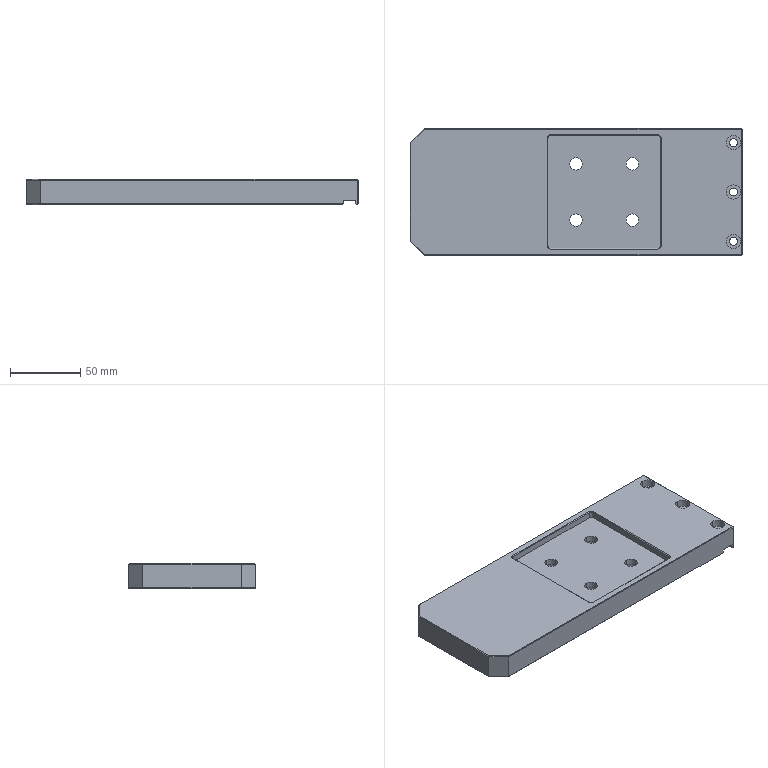NC program | NX | posted with a generic post | part box 235.5 x 90 x 18 mm
Lines 1 to 1608 of 2446:
N10 G17 G21 G94 G90
(DRILLING , TOOL : D6A45)
N12 T01 M6
N14 G54
N16 G17 G0 G90 X111.75 Y35. S5000 M3
N18 G43 Z30. H1
N20 G94 G81 G98 Z-2. F250. R3.
N22 Y0.
N24 Y-35.
N26 X40. Y-20.
N28 X0.
N30 Y20.
N32 X40.
N34 G80
N36 G0 X40. Y20. Z30.
N38 M5
(DRILLING_1 , TOOL : 5.5ZT)
N40 T09 M6
N42 G54
N44 G17 G0 G90 X111.75 Y35. S2000 M3
N46 G43 Z30. H9
N48 G94 G83 G98 Z-21.152 F200. Q2. R3.
N50 Y0.
N52 Y-35.
N54 G80
N56 G0 X111.75 Y-35. Z30.
N58 M5
(DRILLING_1_COPY , TOOL : 9.0ZT)
N60 T16 M6
N62 G54
N64 G17 G0 G90 X0. Y-20. S2000 M3
N66 G43 Z30. H16
N68 G94 G83 G98 Z-22.204 F200. Q2. R3.
N70 Y20.
N72 X40.
N74 Y-20.
N76 G80
N78 G0 X40. Y-20. Z30.
N80 M5
(ZLEVEL_PROFILE , TOOL : D10)
N82 T15 M6
N84 G54
N86 G17 G0 G90 X-122.85 Y10.11 S9500 M3
N88 G43 Z30. H15
N90 Z1.5
N92 G94 G1 Y35.554 Z0.167 F1000.
N94 X-122.49 Y36.963 Z0.09
N96 X-121.748 Y38.215 Z0.014
N98 X-110.965 Y48.998 Z-0.785
N100 X-109.713 Y49.74 Z-0.861
N102 X-108.304 Y50.1 Z-0.938
N104 X-107.75 Z-0.967
N106 X117.25 F3500.
N108 G2 X120.856 Y48.606 R5.1
N110 G1 X121.356 Y48.106
N112 G2 X122.85 Y44.5 R5.1
N114 G1 Y-44.5
N116 G2 X121.356 Y-48.106 R5.1
N118 G1 X120.856 Y-48.606
N120 G2 X117.25 Y-50.1 R5.1
N122 G1 X-107.75
N124 G2 X-111.356 Y-48.606 R5.1
N126 G1 X-121.356 Y-38.606
N128 G2 X-122.85 Y-35. R5.1
N130 G1 Y35.
N132 G2 X-121.356 Y38.606 R5.1
N134 G1 X-111.356 Y48.606
N136 G2 X-107.75 Y50.1 R5.1
N138 G1 X117.25 Z-1.291
N140 X117.75 Y50.075 Z-1.292
N142 X118.245 Y50.002
N144 X118.73 Y49.88 Z-1.293
N146 X119.202 Y49.712 Z-1.294
N148 X119.654 Y49.498 Z-1.295
N150 X120.083 Y49.24
N152 X120.485 Y48.942 Z-1.296
N154 X120.856 Y48.606 Z-1.297
N156 X121.356 Y48.106 Z-1.298
N158 X121.692 Y47.735
N160 X121.99 Y47.333 Z-1.299
N162 X122.248 Y46.904 Z-1.3
N164 X122.462 Y46.452 Z-1.301
N166 X122.63 Y45.98
N168 X122.752 Y45.495 Z-1.302
N170 X122.825 Y45. Z-1.303
N172 X122.85 Y44.5 Z-1.304
N174 Y-44.5 Z-1.432
N176 X122.825 Y-45. Z-1.433
N178 X122.752 Y-45.495
N180 X122.63 Y-45.98 Z-1.434
N182 X122.462 Y-46.452 Z-1.435
N184 X122.248 Y-46.904
N186 X121.99 Y-47.333 Z-1.436
N188 X121.692 Y-47.735 Z-1.437
N190 X121.356 Y-48.106 Z-1.438
N192 X120.856 Y-48.606 Z-1.439
N194 X120.485 Y-48.942
N196 X120.083 Y-49.24 Z-1.44
N198 X119.654 Y-49.498 Z-1.441
N200 X119.202 Y-49.712
N202 X118.73 Y-49.88 Z-1.442
N204 X118.245 Y-50.002 Z-1.443
N206 X117.75 Y-50.075 Z-1.444
N208 X117.25 Y-50.1
N210 X-107.75 Z-1.769
N212 X-108.25 Y-50.075
N214 X-108.745 Y-50.002 Z-1.77
N216 X-109.23 Y-49.88 Z-1.771
N218 X-109.702 Y-49.712 Z-1.772
N220 X-110.154 Y-49.498
N222 X-110.583 Y-49.24 Z-1.773
N224 X-110.985 Y-48.942 Z-1.774
N226 X-111.356 Y-48.606
N228 X-121.356 Y-38.606 Z-1.795
N230 X-121.692 Y-38.235
N232 X-121.99 Y-37.833 Z-1.796
N234 X-122.248 Y-37.404 Z-1.797
N236 X-122.462 Y-36.952 Z-1.798
N238 X-122.63 Y-36.48
N240 X-122.752 Y-35.995 Z-1.799
N242 X-122.825 Y-35.5 Z-1.8
N244 X-122.85 Y-35. Z-1.801
N246 Y35. Z-1.901
N248 X-122.825 Y35.5 Z-1.902
N250 X-122.752 Y35.995 Z-1.903
N252 X-122.63 Y36.48 Z-1.904
N254 X-122.462 Y36.952
N256 X-122.248 Y37.404 Z-1.905
N258 X-121.99 Y37.833 Z-1.906
N260 X-121.692 Y38.235
N262 X-121.356 Y38.606 Z-1.907
N264 X-111.356 Y48.606 Z-1.928
N266 X-110.985 Y48.942
N268 X-110.583 Y49.24 Z-1.929
N270 X-110.154 Y49.498 Z-1.93
N272 X-109.702 Y49.712
N274 X-109.23 Y49.88 Z-1.931
N276 X-108.745 Y50.002 Z-1.932
N278 X-108.25 Y50.075 Z-1.933
N280 X-107.75 Y50.1
N282 X117.25 Z-2.258
N284 X117.75 Y50.075
N286 X118.245 Y50.002 Z-2.259
N288 X118.73 Y49.88 Z-2.26
N290 X119.202 Y49.712 Z-2.261
N292 X119.654 Y49.498
N294 X120.083 Y49.24 Z-2.262
N296 X120.485 Y48.942 Z-2.263
N298 X120.856 Y48.606
N300 X121.356 Y48.106 Z-2.264
N302 X121.692 Y47.735 Z-2.265
N304 X121.99 Y47.333 Z-2.266
N306 X122.248 Y46.904 Z-2.267
N308 X122.462 Y46.452
N310 X122.63 Y45.98 Z-2.268
N312 X122.752 Y45.495 Z-2.269
N314 X122.825 Y45.
N316 X122.85 Y44.5 Z-2.27
N318 Y-44.5 Z-2.398
N320 X122.825 Y-45. Z-2.399
N322 X122.752 Y-45.495 Z-2.4
N324 X122.63 Y-45.98 Z-2.401
N326 X122.462 Y-46.452
N328 X122.248 Y-46.904 Z-2.402
N330 X121.99 Y-47.333 Z-2.403
N332 X121.692 Y-47.735
N334 X121.356 Y-48.106 Z-2.404
N336 X120.856 Y-48.606 Z-2.405
N338 X120.485 Y-48.942 Z-2.406
N340 X120.083 Y-49.24 Z-2.407
N342 X119.654 Y-49.498
N344 X119.202 Y-49.712 Z-2.408
N346 X118.73 Y-49.88 Z-2.409
N348 X118.245 Y-50.002 Z-2.41
N350 X117.75 Y-50.075
N352 X117.25 Y-50.1 Z-2.411
N354 X-107.75 Z-2.735
N356 X-108.25 Y-50.075 Z-2.736
N358 X-108.745 Y-50.002 Z-2.737
N360 X-109.23 Y-49.88
N362 X-109.702 Y-49.712 Z-2.738
N364 X-110.154 Y-49.498 Z-2.739
N366 X-110.583 Y-49.24 Z-2.74
N368 X-110.985 Y-48.942
N370 X-111.356 Y-48.606 Z-2.741
N372 X-121.356 Y-38.606 Z-2.761
N374 X-121.692 Y-38.235 Z-2.762
N376 X-121.99 Y-37.833 Z-2.763
N378 X-122.248 Y-37.404 Z-2.764
N380 X-122.462 Y-36.952
N382 X-122.63 Y-36.48 Z-2.765
N384 X-122.752 Y-35.995 Z-2.766
N386 X-122.825 Y-35.5
N388 X-122.85 Y-35. Z-2.767
N390 Y35. Z-2.868
N392 X-122.825 Y35.5 Z-2.869
N394 X-122.752 Y35.995 Z-2.87
N396 X-122.63 Y36.48
N398 X-122.462 Y36.952 Z-2.871
N400 X-122.248 Y37.404 Z-2.872
N402 X-121.99 Y37.833
N404 X-121.692 Y38.235 Z-2.873
N406 X-121.356 Y38.606 Z-2.874
N408 X-111.356 Y48.606 Z-2.894
N410 X-110.985 Y48.942 Z-2.895
N412 X-110.583 Y49.24 Z-2.896
N414 X-110.154 Y49.498
N416 X-109.702 Y49.712 Z-2.897
N418 X-109.23 Y49.88 Z-2.898
N420 X-108.745 Y50.002 Z-2.899
N422 X-108.25 Y50.075
N424 X-107.75 Y50.1 Z-2.9
N426 X117.25 Z-3.224
N428 X117.75 Y50.075 Z-3.225
N430 X118.245 Y50.002 Z-3.226
N432 X118.73 Y49.88
N434 X119.202 Y49.712 Z-3.227
N436 X119.654 Y49.498 Z-3.228
N438 X120.083 Y49.24 Z-3.229
N440 X120.485 Y48.942
N442 X120.856 Y48.606 Z-3.23
N444 X121.356 Y48.106 Z-3.231
N446 X121.692 Y47.735 Z-3.232
N448 X121.99 Y47.333 Z-3.233
N450 X122.248 Y46.904
N452 X122.462 Y46.452 Z-3.234
N454 X122.63 Y45.98 Z-3.235
N456 X122.752 Y45.495
N458 X122.825 Y45. Z-3.236
N460 X122.85 Y44.5 Z-3.237
N462 Y-44.5 Z-3.365
N464 X122.825 Y-45. Z-3.366
N466 X122.752 Y-45.495 Z-3.367
N468 X122.63 Y-45.98
N470 X122.462 Y-46.452 Z-3.368
N472 X122.248 Y-46.904 Z-3.369
N474 X121.99 Y-47.333
N476 X121.692 Y-47.735 Z-3.37
N478 X121.356 Y-48.106 Z-3.371
N480 X120.856 Y-48.606 Z-3.372
N482 X120.485 Y-48.942 Z-3.373
N484 X120.083 Y-49.24
N486 X119.654 Y-49.498 Z-3.374
N488 X119.202 Y-49.712 Z-3.375
N490 X118.73 Y-49.88 Z-3.376
N492 X118.245 Y-50.002
N494 X117.75 Y-50.075 Z-3.377
N496 X117.25 Y-50.1 Z-3.378
N498 X-107.75 Z-3.702
N500 X-108.25 Y-50.075 Z-3.703
N502 X-108.745 Y-50.002
N504 X-109.23 Y-49.88 Z-3.704
N506 X-109.702 Y-49.712 Z-3.705
N508 X-110.154 Y-49.498 Z-3.706
N510 X-110.583 Y-49.24
N512 X-110.985 Y-48.942 Z-3.707
N514 X-111.356 Y-48.606 Z-3.708
N516 X-121.356 Y-38.606 Z-3.728
N518 X-121.692 Y-38.235 Z-3.729
N520 X-121.99 Y-37.833 Z-3.73
N522 X-122.248 Y-37.404
N524 X-122.462 Y-36.952 Z-3.731
N526 X-122.63 Y-36.48 Z-3.732
N528 X-122.752 Y-35.995
N530 X-122.825 Y-35.5 Z-3.733
N532 X-122.85 Y-35. Z-3.734
N534 Y35. Z-3.835
N536 X-122.825 Y35.5
N538 X-122.752 Y35.995 Z-3.836
N540 X-122.63 Y36.48 Z-3.837
N542 X-122.462 Y36.952 Z-3.838
N544 X-122.248 Y37.404
N546 X-121.99 Y37.833 Z-3.839
N548 X-121.692 Y38.235 Z-3.84
N550 X-121.356 Y38.606 Z-3.841
N552 X-111.356 Y48.606 Z-3.861
N554 X-110.985 Y48.942 Z-3.862
N556 X-110.583 Y49.24
N558 X-110.154 Y49.498 Z-3.863
N560 X-109.702 Y49.712 Z-3.864
N562 X-109.23 Y49.88 Z-3.865
N564 X-108.745 Y50.002
N566 X-108.25 Y50.075 Z-3.866
N568 X-107.75 Y50.1 Z-3.867
N570 X117.25 Z-4.191
N572 X117.75 Y50.075 Z-4.192
N574 X118.245 Y50.002
N576 X118.73 Y49.88 Z-4.193
N578 X119.202 Y49.712 Z-4.194
N580 X119.654 Y49.498 Z-4.195
N582 X120.083 Y49.24
N584 X120.485 Y48.942 Z-4.196
N586 X120.856 Y48.606 Z-4.197
N588 X121.356 Y48.106 Z-4.198
N590 X121.692 Y47.735
N592 X121.99 Y47.333 Z-4.199
N594 X122.248 Y46.904 Z-4.2
N596 X122.462 Y46.452 Z-4.201
N598 X122.63 Y45.98
N600 X122.752 Y45.495 Z-4.202
N602 X122.825 Y45. Z-4.203
N604 X122.85 Y44.5 Z-4.204
N606 Y-44.5 Z-4.332
N608 X122.825 Y-45. Z-4.333
N610 X122.752 Y-45.495
N612 X122.63 Y-45.98 Z-4.334
N614 X122.462 Y-46.452 Z-4.335
N616 X122.248 Y-46.904
N618 X121.99 Y-47.333 Z-4.336
N620 X121.692 Y-47.735 Z-4.337
N622 X121.356 Y-48.106 Z-4.338
N624 X120.856 Y-48.606 Z-4.339
N626 X120.485 Y-48.942
N628 X120.083 Y-49.24 Z-4.34
N630 X119.654 Y-49.498 Z-4.341
N632 X119.202 Y-49.712
N634 X118.73 Y-49.88 Z-4.342
N636 X118.245 Y-50.002 Z-4.343
N638 X117.75 Y-50.075 Z-4.344
N640 X117.25 Y-50.1
N642 X-107.75 Z-4.669
N644 X-108.25 Y-50.075
N646 X-108.745 Y-50.002 Z-4.67
N648 X-109.23 Y-49.88 Z-4.671
N650 X-109.702 Y-49.712 Z-4.672
N652 X-110.154 Y-49.498
N654 X-110.583 Y-49.24 Z-4.673
N656 X-110.985 Y-48.942 Z-4.674
N658 X-111.356 Y-48.606
N660 X-121.356 Y-38.606 Z-4.695
N662 X-121.692 Y-38.235
N664 X-121.99 Y-37.833 Z-4.696
N666 X-122.248 Y-37.404 Z-4.697
N668 X-122.462 Y-36.952 Z-4.698
N670 X-122.63 Y-36.48
N672 X-122.752 Y-35.995 Z-4.699
N674 X-122.825 Y-35.5 Z-4.7
N676 X-122.85 Y-35. Z-4.701
N678 Y35. Z-4.801
N680 X-122.825 Y35.5 Z-4.802
N682 X-122.752 Y35.995 Z-4.803
N684 X-122.63 Y36.48 Z-4.804
N686 X-122.462 Y36.952
N688 X-122.248 Y37.404 Z-4.805
N690 X-121.99 Y37.833 Z-4.806
N692 X-121.692 Y38.235
N694 X-121.356 Y38.606 Z-4.807
N696 X-111.356 Y48.606 Z-4.828
N698 X-110.985 Y48.942
N700 X-110.583 Y49.24 Z-4.829
N702 X-110.154 Y49.498 Z-4.83
N704 X-109.702 Y49.712
N706 X-109.23 Y49.88 Z-4.831
N708 X-108.745 Y50.002 Z-4.832
N710 X-108.25 Y50.075 Z-4.833
N712 X-107.75 Y50.1
N714 X117.25 Z-5.158
N716 X117.75 Y50.075
N718 X118.245 Y50.002 Z-5.159
N720 X118.73 Y49.88 Z-5.16
N722 X119.202 Y49.712 Z-5.161
N724 X119.654 Y49.498
N726 X120.083 Y49.24 Z-5.162
N728 X120.485 Y48.942 Z-5.163
N730 X120.856 Y48.606
N732 X121.356 Y48.106 Z-5.164
N734 X121.692 Y47.735 Z-5.165
N736 X121.99 Y47.333 Z-5.166
N738 X122.248 Y46.904 Z-5.167
N740 X122.462 Y46.452
N742 X122.63 Y45.98 Z-5.168
N744 X122.752 Y45.495 Z-5.169
N746 X122.825 Y45.
N748 X122.85 Y44.5 Z-5.17
N750 Y-44.5 Z-5.298
N752 X122.825 Y-45. Z-5.299
N754 X122.752 Y-45.495 Z-5.3
N756 X122.63 Y-45.98 Z-5.301
N758 X122.462 Y-46.452
N760 X122.248 Y-46.904 Z-5.302
N762 X121.99 Y-47.333 Z-5.303
N764 X121.692 Y-47.735
N766 X121.356 Y-48.106 Z-5.304
N768 X120.856 Y-48.606 Z-5.305
N770 X120.485 Y-48.942 Z-5.306
N772 X120.083 Y-49.24 Z-5.307
N774 X119.654 Y-49.498
N776 X119.202 Y-49.712 Z-5.308
N778 X118.73 Y-49.88 Z-5.309
N780 X118.245 Y-50.002 Z-5.31
N782 X117.75 Y-50.075
N784 X117.25 Y-50.1 Z-5.311
N786 X-107.75 Z-5.635
N788 X-108.25 Y-50.075 Z-5.636
N790 X-108.745 Y-50.002 Z-5.637
N792 X-109.23 Y-49.88
N794 X-109.702 Y-49.712 Z-5.638
N796 X-110.154 Y-49.498 Z-5.639
N798 X-110.583 Y-49.24 Z-5.64
N800 X-110.985 Y-48.942
N802 X-111.356 Y-48.606 Z-5.641
N804 X-121.356 Y-38.606 Z-5.661
N806 X-121.692 Y-38.235 Z-5.662
N808 X-121.99 Y-37.833 Z-5.663
N810 X-122.248 Y-37.404 Z-5.664
N812 X-122.462 Y-36.952
N814 X-122.63 Y-36.48 Z-5.665
N816 X-122.752 Y-35.995 Z-5.666
N818 X-122.825 Y-35.5
N820 X-122.85 Y-35. Z-5.667
N822 Y35. Z-5.768
N824 X-122.825 Y35.5 Z-5.769
N826 X-122.752 Y35.995 Z-5.77
N828 X-122.63 Y36.48
N830 X-122.462 Y36.952 Z-5.771
N832 X-122.248 Y37.404 Z-5.772
N834 X-121.99 Y37.833
N836 X-121.692 Y38.235 Z-5.773
N838 X-121.356 Y38.606 Z-5.774
N840 X-111.356 Y48.606 Z-5.794
N842 X-110.985 Y48.942 Z-5.795
N844 X-110.583 Y49.24 Z-5.796
N846 X-110.154 Y49.498
N848 X-109.702 Y49.712 Z-5.797
N850 X-109.23 Y49.88 Z-5.798
N852 X-108.745 Y50.002 Z-5.799
N854 X-108.25 Y50.075
N856 X-107.75 Y50.1 Z-5.8
N858 X117.25 Z-6.124
N860 X117.75 Y50.075 Z-6.125
N862 X118.245 Y50.002 Z-6.126
N864 X118.73 Y49.88
N866 X119.202 Y49.712 Z-6.127
N868 X119.654 Y49.498 Z-6.128
N870 X120.083 Y49.24 Z-6.129
N872 X120.485 Y48.942
N874 X120.856 Y48.606 Z-6.13
N876 X121.356 Y48.106 Z-6.131
N878 X121.692 Y47.735 Z-6.132
N880 X121.99 Y47.333 Z-6.133
N882 X122.248 Y46.904
N884 X122.462 Y46.452 Z-6.134
N886 X122.63 Y45.98 Z-6.135
N888 X122.752 Y45.495
N890 X122.825 Y45. Z-6.136
N892 X122.85 Y44.5 Z-6.137
N894 Y-44.5 Z-6.265
N896 X122.825 Y-45. Z-6.266
N898 X122.752 Y-45.495 Z-6.267
N900 X122.63 Y-45.98
N902 X122.462 Y-46.452 Z-6.268
N904 X122.248 Y-46.904 Z-6.269
N906 X121.99 Y-47.333
N908 X121.692 Y-47.735 Z-6.27
N910 X121.356 Y-48.106 Z-6.271
N912 X120.856 Y-48.606 Z-6.272
N914 X120.485 Y-48.942 Z-6.273
N916 X120.083 Y-49.24
N918 X119.654 Y-49.498 Z-6.274
N920 X119.202 Y-49.712 Z-6.275
N922 X118.73 Y-49.88 Z-6.276
N924 X118.245 Y-50.002
N926 X117.75 Y-50.075 Z-6.277
N928 X117.25 Y-50.1 Z-6.278
N930 X-107.75 Z-6.602
N932 X-108.25 Y-50.075 Z-6.603
N934 X-108.745 Y-50.002
N936 X-109.23 Y-49.88 Z-6.604
N938 X-109.702 Y-49.712 Z-6.605
N940 X-110.154 Y-49.498 Z-6.606
N942 X-110.583 Y-49.24
N944 X-110.985 Y-48.942 Z-6.607
N946 X-111.356 Y-48.606 Z-6.608
N948 X-121.356 Y-38.606 Z-6.628
N950 X-121.692 Y-38.235 Z-6.629
N952 X-121.99 Y-37.833 Z-6.63
N954 X-122.248 Y-37.404
N956 X-122.462 Y-36.952 Z-6.631
N958 X-122.63 Y-36.48 Z-6.632
N960 X-122.752 Y-35.995
N962 X-122.825 Y-35.5 Z-6.633
N964 X-122.85 Y-35. Z-6.634
N966 Y35. Z-6.735
N968 X-122.825 Y35.5
N970 X-122.752 Y35.995 Z-6.736
N972 X-122.63 Y36.48 Z-6.737
N974 X-122.462 Y36.952 Z-6.738
N976 X-122.248 Y37.404
N978 X-121.99 Y37.833 Z-6.739
N980 X-121.692 Y38.235 Z-6.74
N982 X-121.356 Y38.606 Z-6.741
N984 X-111.356 Y48.606 Z-6.761
N986 X-110.985 Y48.942 Z-6.762
N988 X-110.583 Y49.24
N990 X-110.154 Y49.498 Z-6.763
N992 X-109.702 Y49.712 Z-6.764
N994 X-109.23 Y49.88 Z-6.765
N996 X-108.745 Y50.002
N998 X-108.25 Y50.075 Z-6.766
N1000 X-107.75 Y50.1 Z-6.767
N1002 X117.25 Z-7.091
N1004 X117.75 Y50.075 Z-7.092
N1006 X118.245 Y50.002
N1008 X118.73 Y49.88 Z-7.093
N1010 X119.202 Y49.712 Z-7.094
N1012 X119.654 Y49.498 Z-7.095
N1014 X120.083 Y49.24
N1016 X120.485 Y48.942 Z-7.096
N1018 X120.856 Y48.606 Z-7.097
N1020 X121.356 Y48.106 Z-7.098
N1022 X121.692 Y47.735
N1024 X121.99 Y47.333 Z-7.099
N1026 X122.248 Y46.904 Z-7.1
N1028 X122.462 Y46.452 Z-7.101
N1030 X122.63 Y45.98
N1032 X122.752 Y45.495 Z-7.102
N1034 X122.825 Y45. Z-7.103
N1036 X122.85 Y44.5 Z-7.104
N1038 Y-44.5 Z-7.232
N1040 X122.825 Y-45. Z-7.233
N1042 X122.752 Y-45.495
N1044 X122.63 Y-45.98 Z-7.234
N1046 X122.462 Y-46.452 Z-7.235
N1048 X122.248 Y-46.904
N1050 X121.99 Y-47.333 Z-7.236
N1052 X121.692 Y-47.735 Z-7.237
N1054 X121.356 Y-48.106 Z-7.238
N1056 X120.856 Y-48.606 Z-7.239
N1058 X120.485 Y-48.942
N1060 X120.083 Y-49.24 Z-7.24
N1062 X119.654 Y-49.498 Z-7.241
N1064 X119.202 Y-49.712
N1066 X118.73 Y-49.88 Z-7.242
N1068 X118.245 Y-50.002 Z-7.243
N1070 X117.75 Y-50.075 Z-7.244
N1072 X117.25 Y-50.1
N1074 X-107.75 Z-7.569
N1076 X-108.25 Y-50.075
N1078 X-108.745 Y-50.002 Z-7.57
N1080 X-109.23 Y-49.88 Z-7.571
N1082 X-109.702 Y-49.712 Z-7.572
N1084 X-110.154 Y-49.498
N1086 X-110.583 Y-49.24 Z-7.573
N1088 X-110.985 Y-48.942 Z-7.574
N1090 X-111.356 Y-48.606
N1092 X-121.356 Y-38.606 Z-7.595
N1094 X-121.692 Y-38.235
N1096 X-121.99 Y-37.833 Z-7.596
N1098 X-122.248 Y-37.404 Z-7.597
N1100 X-122.462 Y-36.952 Z-7.598
N1102 X-122.63 Y-36.48
N1104 X-122.752 Y-35.995 Z-7.599
N1106 X-122.825 Y-35.5 Z-7.6
N1108 X-122.85 Y-35. Z-7.601
N1110 Y35. Z-7.701
N1112 X-122.825 Y35.5 Z-7.702
N1114 X-122.752 Y35.995 Z-7.703
N1116 X-122.63 Y36.48 Z-7.704
N1118 X-122.462 Y36.952
N1120 X-122.248 Y37.404 Z-7.705
N1122 X-121.99 Y37.833 Z-7.706
N1124 X-121.692 Y38.235
N1126 X-121.356 Y38.606 Z-7.707
N1128 X-111.356 Y48.606 Z-7.728
N1130 X-110.985 Y48.942
N1132 X-110.583 Y49.24 Z-7.729
N1134 X-110.154 Y49.498 Z-7.73
N1136 X-109.702 Y49.712
N1138 X-109.23 Y49.88 Z-7.731
N1140 X-108.745 Y50.002 Z-7.732
N1142 X-108.25 Y50.075 Z-7.733
N1144 X-107.75 Y50.1
N1146 X117.25 Z-8.058
N1148 X117.75 Y50.075
N1150 X118.245 Y50.002 Z-8.059
N1152 X118.73 Y49.88 Z-8.06
N1154 X119.202 Y49.712 Z-8.061
N1156 X119.654 Y49.498
N1158 X120.083 Y49.24 Z-8.062
N1160 X120.485 Y48.942 Z-8.063
N1162 X120.856 Y48.606
N1164 X121.356 Y48.106 Z-8.064
N1166 X121.692 Y47.735 Z-8.065
N1168 X121.99 Y47.333 Z-8.066
N1170 X122.248 Y46.904 Z-8.067
N1172 X122.462 Y46.452
N1174 X122.63 Y45.98 Z-8.068
N1176 X122.752 Y45.495 Z-8.069
N1178 X122.825 Y45.
N1180 X122.85 Y44.5 Z-8.07
N1182 Y-44.5 Z-8.198
N1184 X122.825 Y-45. Z-8.199
N1186 X122.752 Y-45.495 Z-8.2
N1188 X122.63 Y-45.98 Z-8.201
N1190 X122.462 Y-46.452
N1192 X122.248 Y-46.904 Z-8.202
N1194 X121.99 Y-47.333 Z-8.203
N1196 X121.692 Y-47.735
N1198 X121.356 Y-48.106 Z-8.204
N1200 X120.856 Y-48.606 Z-8.205
N1202 X120.485 Y-48.942 Z-8.206
N1204 X120.083 Y-49.24 Z-8.207
N1206 X119.654 Y-49.498
N1208 X119.202 Y-49.712 Z-8.208
N1210 X118.73 Y-49.88 Z-8.209
N1212 X118.245 Y-50.002 Z-8.21
N1214 X117.75 Y-50.075
N1216 X117.25 Y-50.1 Z-8.211
N1218 X-107.75 Z-8.535
N1220 X-108.25 Y-50.075 Z-8.536
N1222 X-108.745 Y-50.002 Z-8.537
N1224 X-109.23 Y-49.88
N1226 X-109.702 Y-49.712 Z-8.538
N1228 X-110.154 Y-49.498 Z-8.539
N1230 X-110.583 Y-49.24 Z-8.54
N1232 X-110.985 Y-48.942
N1234 X-111.356 Y-48.606 Z-8.541
N1236 X-121.356 Y-38.606 Z-8.561
N1238 X-121.692 Y-38.235 Z-8.562
N1240 X-121.99 Y-37.833 Z-8.563
N1242 X-122.248 Y-37.404 Z-8.564
N1244 X-122.462 Y-36.952
N1246 X-122.63 Y-36.48 Z-8.565
N1248 X-122.752 Y-35.995 Z-8.566
N1250 X-122.825 Y-35.5
N1252 X-122.85 Y-35. Z-8.567
N1254 Y35. Z-8.668
N1256 X-122.825 Y35.5 Z-8.669
N1258 X-122.752 Y35.995 Z-8.67
N1260 X-122.63 Y36.48
N1262 X-122.462 Y36.952 Z-8.671
N1264 X-122.248 Y37.404 Z-8.672
N1266 X-121.99 Y37.833
N1268 X-121.692 Y38.235 Z-8.673
N1270 X-121.356 Y38.606 Z-8.674
N1272 X-111.356 Y48.606 Z-8.694
N1274 X-110.985 Y48.942 Z-8.695
N1276 X-110.583 Y49.24 Z-8.696
N1278 X-110.154 Y49.498
N1280 X-109.702 Y49.712 Z-8.697
N1282 X-109.23 Y49.88 Z-8.698
N1284 X-108.745 Y50.002 Z-8.699
N1286 X-108.25 Y50.075
N1288 X-107.75 Y50.1 Z-8.7
N1290 X117.25 Z-9.024
N1292 X117.75 Y50.075 Z-9.025
N1294 X118.245 Y50.002 Z-9.026
N1296 X118.73 Y49.88
N1298 X119.202 Y49.712 Z-9.027
N1300 X119.654 Y49.498 Z-9.028
N1302 X120.083 Y49.24 Z-9.029
N1304 X120.485 Y48.942
N1306 X120.856 Y48.606 Z-9.03
N1308 X121.356 Y48.106 Z-9.031
N1310 X121.692 Y47.735 Z-9.032
N1312 X121.99 Y47.333 Z-9.033
N1314 X122.248 Y46.904
N1316 X122.462 Y46.452 Z-9.034
N1318 X122.63 Y45.98 Z-9.035
N1320 X122.752 Y45.495
N1322 X122.825 Y45. Z-9.036
N1324 X122.85 Y44.5 Z-9.037
N1326 Y-44.5 Z-9.165
N1328 X122.825 Y-45. Z-9.166
N1330 X122.752 Y-45.495 Z-9.167
N1332 X122.63 Y-45.98
N1334 X122.462 Y-46.452 Z-9.168
N1336 X122.248 Y-46.904 Z-9.169
N1338 X121.99 Y-47.333
N1340 X121.692 Y-47.735 Z-9.17
N1342 X121.356 Y-48.106 Z-9.171
N1344 X120.856 Y-48.606 Z-9.172
N1346 X120.485 Y-48.942 Z-9.173
N1348 X120.083 Y-49.24
N1350 X119.654 Y-49.498 Z-9.174
N1352 X119.202 Y-49.712 Z-9.175
N1354 X118.73 Y-49.88 Z-9.176
N1356 X118.245 Y-50.002
N1358 X117.75 Y-50.075 Z-9.177
N1360 X117.25 Y-50.1 Z-9.178
N1362 X-107.75 Z-9.502
N1364 X-108.25 Y-50.075 Z-9.503
N1366 X-108.745 Y-50.002
N1368 X-109.23 Y-49.88 Z-9.504
N1370 X-109.702 Y-49.712 Z-9.505
N1372 X-110.154 Y-49.498 Z-9.506
N1374 X-110.583 Y-49.24
N1376 X-110.985 Y-48.942 Z-9.507
N1378 X-111.356 Y-48.606 Z-9.508
N1380 X-121.356 Y-38.606 Z-9.528
N1382 X-121.692 Y-38.235 Z-9.529
N1384 X-121.99 Y-37.833 Z-9.53
N1386 X-122.248 Y-37.404
N1388 X-122.462 Y-36.952 Z-9.531
N1390 X-122.63 Y-36.48 Z-9.532
N1392 X-122.752 Y-35.995
N1394 X-122.825 Y-35.5 Z-9.533
N1396 X-122.85 Y-35. Z-9.534
N1398 Y35. Z-9.635
N1400 X-122.825 Y35.5
N1402 X-122.752 Y35.995 Z-9.636
N1404 X-122.63 Y36.48 Z-9.637
N1406 X-122.462 Y36.952 Z-9.638
N1408 X-122.248 Y37.404
N1410 X-121.99 Y37.833 Z-9.639
N1412 X-121.692 Y38.235 Z-9.64
N1414 X-121.356 Y38.606 Z-9.641
N1416 X-111.356 Y48.606 Z-9.661
N1418 X-110.985 Y48.942 Z-9.662
N1420 X-110.583 Y49.24
N1422 X-110.154 Y49.498 Z-9.663
N1424 X-109.702 Y49.712 Z-9.664
N1426 X-109.23 Y49.88 Z-9.665
N1428 X-108.745 Y50.002
N1430 X-108.25 Y50.075 Z-9.666
N1432 X-107.75 Y50.1 Z-9.667
N1434 X117.25 Z-9.991
N1436 X117.75 Y50.075 Z-9.992
N1438 X118.245 Y50.002
N1440 X118.73 Y49.88 Z-9.993
N1442 X119.202 Y49.712 Z-9.994
N1444 X119.654 Y49.498 Z-9.995
N1446 X120.083 Y49.24
N1448 X120.485 Y48.942 Z-9.996
N1450 X120.856 Y48.606 Z-9.997
N1452 X121.356 Y48.106 Z-9.998
N1454 X121.692 Y47.735
N1456 X121.99 Y47.333 Z-9.999
N1458 X122.248 Y46.904 Z-10.
N1460 X122.462 Y46.452 Z-10.001
N1462 X122.63 Y45.98
N1464 X122.752 Y45.495 Z-10.002
N1466 X122.825 Y45. Z-10.003
N1468 X122.85 Y44.5 Z-10.004
N1470 Y-44.5 Z-10.132
N1472 X122.825 Y-45. Z-10.133
N1474 X122.752 Y-45.495
N1476 X122.63 Y-45.98 Z-10.134
N1478 X122.462 Y-46.452 Z-10.135
N1480 X122.248 Y-46.904
N1482 X121.99 Y-47.333 Z-10.136
N1484 X121.692 Y-47.735 Z-10.137
N1486 X121.356 Y-48.106 Z-10.138
N1488 X120.856 Y-48.606 Z-10.139
N1490 X120.485 Y-48.942
N1492 X120.083 Y-49.24 Z-10.14
N1494 X119.654 Y-49.498 Z-10.141
N1496 X119.202 Y-49.712
N1498 X118.73 Y-49.88 Z-10.142
N1500 X118.245 Y-50.002 Z-10.143
N1502 X117.75 Y-50.075 Z-10.144
N1504 X117.25 Y-50.1
N1506 X-107.75 Z-10.469
N1508 X-108.25 Y-50.075
N1510 X-108.745 Y-50.002 Z-10.47
N1512 X-109.23 Y-49.88 Z-10.471
N1514 X-109.702 Y-49.712 Z-10.472
N1516 X-110.154 Y-49.498
N1518 X-110.583 Y-49.24 Z-10.473
N1520 X-110.985 Y-48.942 Z-10.474
N1522 X-111.356 Y-48.606
N1524 X-121.356 Y-38.606 Z-10.495
N1526 X-121.692 Y-38.235
N1528 X-121.99 Y-37.833 Z-10.496
N1530 X-122.248 Y-37.404 Z-10.497
N1532 X-122.462 Y-36.952 Z-10.498
N1534 X-122.63 Y-36.48
N1536 X-122.752 Y-35.995 Z-10.499
N1538 X-122.825 Y-35.5 Z-10.5
N1540 X-122.85 Y-35. Z-10.501
N1542 Y35. Z-10.601
N1544 X-122.825 Y35.5 Z-10.602
N1546 X-122.752 Y35.995 Z-10.603
N1548 X-122.63 Y36.48 Z-10.604
N1550 X-122.462 Y36.952
N1552 X-122.248 Y37.404 Z-10.605
N1554 X-121.99 Y37.833 Z-10.606
N1556 X-121.692 Y38.235
N1558 X-121.356 Y38.606 Z-10.607
N1560 X-111.356 Y48.606 Z-10.628
N1562 X-110.985 Y48.942
N1564 X-110.583 Y49.24 Z-10.629
N1566 X-110.154 Y49.498 Z-10.63
N1568 X-109.702 Y49.712
N1570 X-109.23 Y49.88 Z-10.631
N1572 X-108.745 Y50.002 Z-10.632
N1574 X-108.25 Y50.075 Z-10.633
N1576 X-107.75 Y50.1
N1578 X117.25 Z-10.958
N1580 X117.75 Y50.075
N1582 X118.245 Y50.002 Z-10.959
N1584 X118.73 Y49.88 Z-10.96
N1586 X119.202 Y49.712 Z-10.961
N1588 X119.654 Y49.498
N1590 X120.083 Y49.24 Z-10.962
N1592 X120.485 Y48.942 Z-10.963
N1594 X120.856 Y48.606
N1596 X121.356 Y48.106 Z-10.964
N1598 X121.692 Y47.735 Z-10.965
N1600 X121.99 Y47.333 Z-10.966
N1602 X122.248 Y46.904 Z-10.967
N1604 X122.462 Y46.452
N1606 X122.63 Y45.98 Z-10.968
N1608 X122.752 Y45.495 Z-10.969
N1610 X122.825 Y45.
N1612 X122.85 Y44.5 Z-10.97
N1614 Y-44.5 Z-11.098
N1616 X122.825 Y-45. Z-11.099
N1618 X122.752 Y-45.495 Z-11.1
N1620 X122.63 Y-45.98 Z-11.101
N1622 X122.462 Y-46.452
N1624 X122.248 Y-46.904 Z-11.102
N1626 X121.99 Y-47.333 Z-11.103
N1628 X121.692 Y-47.735
N1630 X121.356 Y-48.106 Z-11.104
N1632 X120.856 Y-48.606 Z-11.105
N1634 X120.485 Y-48.942 Z-11.106
N1636 X120.083 Y-49.24 Z-11.107
N1638 X119.654 Y-49.498
N1640 X119.202 Y-49.712 Z-11.108
N1642 X118.73 Y-49.88 Z-11.109
N1644 X118.245 Y-50.002 Z-11.11
N1646 X117.75 Y-50.075
N1648 X117.25 Y-50.1 Z-11.111
N1650 X-107.75 Z-11.435
N1652 X-108.25 Y-50.075 Z-11.436
N1654 X-108.745 Y-50.002 Z-11.437
N1656 X-109.23 Y-49.88
N1658 X-109.702 Y-49.712 Z-11.438
N1660 X-110.154 Y-49.498 Z-11.439
N1662 X-110.583 Y-49.24 Z-11.44
N1664 X-110.985 Y-48.942
N1666 X-111.356 Y-48.606 Z-11.441
N1668 X-121.356 Y-38.606 Z-11.461
N1670 X-121.692 Y-38.235 Z-11.462
N1672 X-121.99 Y-37.833 Z-11.463
N1674 X-122.248 Y-37.404 Z-11.464
N1676 X-122.462 Y-36.952
N1678 X-122.63 Y-36.48 Z-11.465
N1680 X-122.752 Y-35.995 Z-11.466
N1682 X-122.825 Y-35.5
N1684 X-122.85 Y-35. Z-11.467
N1686 Y35. Z-11.568
N1688 X-122.825 Y35.5 Z-11.569
N1690 X-122.752 Y35.995 Z-11.57
N1692 X-122.63 Y36.48
N1694 X-122.462 Y36.952 Z-11.571
N1696 X-122.248 Y37.404 Z-11.572
N1698 X-121.99 Y37.833
N1700 X-121.692 Y38.235 Z-11.573
N1702 X-121.356 Y38.606 Z-11.574
N1704 X-111.356 Y48.606 Z-11.594
N1706 X-110.985 Y48.942 Z-11.595
N1708 X-110.583 Y49.24 Z-11.596
N1710 X-110.154 Y49.498
N1712 X-109.702 Y49.712 Z-11.597
N1714 X-109.23 Y49.88 Z-11.598
N1716 X-108.745 Y50.002 Z-11.599
N1718 X-108.25 Y50.075
N1720 X-107.75 Y50.1 Z-11.6
N1722 X117.25 Z-11.924
N1724 X117.75 Y50.075 Z-11.925
N1726 X118.245 Y50.002 Z-11.926
N1728 X118.73 Y49.88
N1730 X119.202 Y49.712 Z-11.927
N1732 X119.654 Y49.498 Z-11.928
N1734 X120.083 Y49.24 Z-11.929
N1736 X120.485 Y48.942
N1738 X120.856 Y48.606 Z-11.93
N1740 X121.356 Y48.106 Z-11.931
N1742 X121.692 Y47.735 Z-11.932
N1744 X121.99 Y47.333 Z-11.933
N1746 X122.248 Y46.904
N1748 X122.462 Y46.452 Z-11.934
N1750 X122.63 Y45.98 Z-11.935
N1752 X122.752 Y45.495
N1754 X122.825 Y45. Z-11.936
N1756 X122.85 Y44.5 Z-11.937
N1758 Y-44.5 Z-12.065
N1760 X122.825 Y-45. Z-12.066
N1762 X122.752 Y-45.495 Z-12.067
N1764 X122.63 Y-45.98
N1766 X122.462 Y-46.452 Z-12.068
N1768 X122.248 Y-46.904 Z-12.069
N1770 X121.99 Y-47.333
N1772 X121.692 Y-47.735 Z-12.07
N1774 X121.356 Y-48.106 Z-12.071
N1776 X120.856 Y-48.606 Z-12.072
N1778 X120.485 Y-48.942 Z-12.073
N1780 X120.083 Y-49.24
N1782 X119.654 Y-49.498 Z-12.074
N1784 X119.202 Y-49.712 Z-12.075
N1786 X118.73 Y-49.88 Z-12.076
N1788 X118.245 Y-50.002
N1790 X117.75 Y-50.075 Z-12.077
N1792 X117.25 Y-50.1 Z-12.078
N1794 X-107.75 Z-12.402
N1796 X-108.25 Y-50.075 Z-12.403
N1798 X-108.745 Y-50.002
N1800 X-109.23 Y-49.88 Z-12.404
N1802 X-109.702 Y-49.712 Z-12.405
N1804 X-110.154 Y-49.498 Z-12.406
N1806 X-110.583 Y-49.24
N1808 X-110.985 Y-48.942 Z-12.407
N1810 X-111.356 Y-48.606 Z-12.408
N1812 X-121.356 Y-38.606 Z-12.428
N1814 X-121.692 Y-38.235 Z-12.429
N1816 X-121.99 Y-37.833 Z-12.43
N1818 X-122.248 Y-37.404
N1820 X-122.462 Y-36.952 Z-12.431
N1822 X-122.63 Y-36.48 Z-12.432
N1824 X-122.752 Y-35.995
N1826 X-122.825 Y-35.5 Z-12.433
N1828 X-122.85 Y-35. Z-12.434
N1830 Y35. Z-12.535
N1832 X-122.825 Y35.5
N1834 X-122.752 Y35.995 Z-12.536
N1836 X-122.63 Y36.48 Z-12.537
N1838 X-122.462 Y36.952 Z-12.538
N1840 X-122.248 Y37.404
N1842 X-121.99 Y37.833 Z-12.539
N1844 X-121.692 Y38.235 Z-12.54
N1846 X-121.356 Y38.606 Z-12.541
N1848 X-111.356 Y48.606 Z-12.561
N1850 X-110.985 Y48.942 Z-12.562
N1852 X-110.583 Y49.24
N1854 X-110.154 Y49.498 Z-12.563
N1856 X-109.702 Y49.712 Z-12.564
N1858 X-109.23 Y49.88 Z-12.565
N1860 X-108.745 Y50.002
N1862 X-108.25 Y50.075 Z-12.566
N1864 X-107.75 Y50.1 Z-12.567
N1866 X117.25 Z-12.891
N1868 X117.75 Y50.075 Z-12.892
N1870 X118.245 Y50.002
N1872 X118.73 Y49.88 Z-12.893
N1874 X119.202 Y49.712 Z-12.894
N1876 X119.654 Y49.498 Z-12.895
N1878 X120.083 Y49.24
N1880 X120.485 Y48.942 Z-12.896
N1882 X120.856 Y48.606 Z-12.897
N1884 X121.356 Y48.106 Z-12.898
N1886 X121.692 Y47.735
N1888 X121.99 Y47.333 Z-12.899
N1890 X122.248 Y46.904 Z-12.9
N1892 X122.462 Y46.452 Z-12.901
N1894 X122.63 Y45.98
N1896 X122.752 Y45.495 Z-12.902
N1898 X122.825 Y45. Z-12.903
N1900 X122.85 Y44.5 Z-12.904
N1902 Y-44.5 Z-13.032
N1904 X122.825 Y-45. Z-13.033
N1906 X122.752 Y-45.495
N1908 X122.63 Y-45.98 Z-13.034
N1910 X122.462 Y-46.452 Z-13.035
N1912 X122.248 Y-46.904
N1914 X121.99 Y-47.333 Z-13.036
N1916 X121.692 Y-47.735 Z-13.037
N1918 X121.356 Y-48.106 Z-13.038
N1920 X120.856 Y-48.606 Z-13.039
N1922 X120.485 Y-48.942
N1924 X120.083 Y-49.24 Z-13.04
N1926 X119.654 Y-49.498 Z-13.041
N1928 X119.202 Y-49.712
N1930 X118.73 Y-49.88 Z-13.042
N1932 X118.245 Y-50.002 Z-13.043
N1934 X117.75 Y-50.075 Z-13.044
N1936 X117.25 Y-50.1
N1938 X-107.75 Z-13.369
N1940 X-108.25 Y-50.075
N1942 X-108.745 Y-50.002 Z-13.37
N1944 X-109.23 Y-49.88 Z-13.371
N1946 X-109.702 Y-49.712 Z-13.372
N1948 X-110.154 Y-49.498
N1950 X-110.583 Y-49.24 Z-13.373
N1952 X-110.985 Y-48.942 Z-13.374
N1954 X-111.356 Y-48.606
N1956 X-121.356 Y-38.606 Z-13.395
N1958 X-121.692 Y-38.235
N1960 X-121.99 Y-37.833 Z-13.396
N1962 X-122.248 Y-37.404 Z-13.397
N1964 X-122.462 Y-36.952 Z-13.398
N1966 X-122.63 Y-36.48
N1968 X-122.752 Y-35.995 Z-13.399
N1970 X-122.825 Y-35.5 Z-13.4
N1972 X-122.85 Y-35. Z-13.401
N1974 Y35. Z-13.501
N1976 X-122.825 Y35.5 Z-13.502
N1978 X-122.752 Y35.995 Z-13.503
N1980 X-122.63 Y36.48 Z-13.504
N1982 X-122.462 Y36.952
N1984 X-122.248 Y37.404 Z-13.505
N1986 X-121.99 Y37.833 Z-13.506
N1988 X-121.692 Y38.235
N1990 X-121.356 Y38.606 Z-13.507
N1992 X-111.356 Y48.606 Z-13.528
N1994 X-110.985 Y48.942
N1996 X-110.583 Y49.24 Z-13.529
N1998 X-110.154 Y49.498 Z-13.53
N2000 X-109.702 Y49.712
N2002 X-109.23 Y49.88 Z-13.531
N2004 X-108.745 Y50.002 Z-13.532
N2006 X-108.25 Y50.075 Z-13.533
N2008 X-107.75 Y50.1
N2010 X117.25 Z-13.858
N2012 X117.75 Y50.075
N2014 X118.245 Y50.002 Z-13.859
N2016 X118.73 Y49.88 Z-13.86
N2018 X119.202 Y49.712 Z-13.861
N2020 X119.654 Y49.498
N2022 X120.083 Y49.24 Z-13.862
N2024 X120.485 Y48.942 Z-13.863
N2026 X120.856 Y48.606
N2028 X121.356 Y48.106 Z-13.864
N2030 X121.692 Y47.735 Z-13.865
N2032 X121.99 Y47.333 Z-13.866
N2034 X122.248 Y46.904 Z-13.867
N2036 X122.462 Y46.452
N2038 X122.63 Y45.98 Z-13.868
N2040 X122.752 Y45.495 Z-13.869
N2042 X122.825 Y45.
N2044 X122.85 Y44.5 Z-13.87
N2046 Y-44.5 Z-13.998
N2048 X122.825 Y-45. Z-13.999
N2050 X122.752 Y-45.495 Z-14.
N2052 X122.63 Y-45.98 Z-14.001
N2054 X122.462 Y-46.452
N2056 X122.248 Y-46.904 Z-14.002
N2058 X121.99 Y-47.333 Z-14.003
N2060 X121.692 Y-47.735
N2062 X121.356 Y-48.106 Z-14.004
N2064 X120.856 Y-48.606 Z-14.005
N2066 X120.485 Y-48.942 Z-14.006
N2068 X120.083 Y-49.24 Z-14.007
N2070 X119.654 Y-49.498
N2072 X119.202 Y-49.712 Z-14.008
N2074 X118.73 Y-49.88 Z-14.009
N2076 X118.245 Y-50.002 Z-14.01
N2078 X117.75 Y-50.075
N2080 X117.25 Y-50.1 Z-14.011
N2082 X-107.75 Z-14.335
N2084 X-108.25 Y-50.075 Z-14.336
N2086 X-108.745 Y-50.002 Z-14.337
N2088 X-109.23 Y-49.88
N2090 X-109.702 Y-49.712 Z-14.338
N2092 X-110.154 Y-49.498 Z-14.339
N2094 X-110.583 Y-49.24 Z-14.34
N2096 X-110.985 Y-48.942
N2098 X-111.356 Y-48.606 Z-14.341
N2100 X-121.356 Y-38.606 Z-14.361
N2102 X-121.692 Y-38.235 Z-14.362
N2104 X-121.99 Y-37.833 Z-14.363
N2106 X-122.248 Y-37.404 Z-14.364
N2108 X-122.462 Y-36.952
N2110 X-122.63 Y-36.48 Z-14.365
N2112 X-122.752 Y-35.995 Z-14.366
N2114 X-122.825 Y-35.5
N2116 X-122.85 Y-35. Z-14.367
N2118 Y35. Z-14.468
N2120 X-122.825 Y35.5 Z-14.469
N2122 X-122.752 Y35.995 Z-14.47
N2124 X-122.63 Y36.48
N2126 X-122.462 Y36.952 Z-14.471
N2128 X-122.248 Y37.404 Z-14.472
N2130 X-121.99 Y37.833
N2132 X-121.692 Y38.235 Z-14.473
N2134 X-121.356 Y38.606 Z-14.474
N2136 X-111.356 Y48.606 Z-14.494
N2138 X-110.985 Y48.942 Z-14.495
N2140 X-110.583 Y49.24 Z-14.496
N2142 X-110.154 Y49.498
N2144 X-109.702 Y49.712 Z-14.497
N2146 X-109.23 Y49.88 Z-14.498
N2148 X-108.745 Y50.002 Z-14.499
N2150 X-108.25 Y50.075
N2152 X-107.75 Y50.1 Z-14.5
N2154 X117.25 Z-14.824
N2156 X117.75 Y50.075 Z-14.825
N2158 X118.245 Y50.002 Z-14.826
N2160 X118.73 Y49.88
N2162 X119.202 Y49.712 Z-14.827
N2164 X119.654 Y49.498 Z-14.828
N2166 X120.083 Y49.24 Z-14.829
N2168 X120.485 Y48.942
N2170 X120.856 Y48.606 Z-14.83
N2172 X121.356 Y48.106 Z-14.831
N2174 X121.692 Y47.735 Z-14.832
N2176 X121.99 Y47.333 Z-14.833
N2178 X122.248 Y46.904
N2180 X122.462 Y46.452 Z-14.834
N2182 X122.63 Y45.98 Z-14.835
N2184 X122.752 Y45.495
N2186 X122.825 Y45. Z-14.836
N2188 X122.85 Y44.5 Z-14.837
N2190 Y-44.5 Z-14.965
N2192 X122.825 Y-45. Z-14.966
N2194 X122.752 Y-45.495 Z-14.967
N2196 X122.63 Y-45.98
N2198 X122.462 Y-46.452 Z-14.968
N2200 X122.248 Y-46.904 Z-14.969
N2202 X121.99 Y-47.333
N2204 X121.692 Y-47.735 Z-14.97
N2206 X121.356 Y-48.106 Z-14.971
N2208 X120.856 Y-48.606 Z-14.972
N2210 X120.485 Y-48.942 Z-14.973
N2212 X120.083 Y-49.24
N2214 X119.654 Y-49.498 Z-14.974
N2216 X119.202 Y-49.712 Z-14.975
N2218 X118.73 Y-49.88 Z-14.976
N2220 X118.245 Y-50.002
N2222 X117.75 Y-50.075 Z-14.977
N2224 X117.25 Y-50.1 Z-14.978
N2226 X-107.75 Z-15.302
N2228 X-108.25 Y-50.075 Z-15.303
N2230 X-108.745 Y-50.002
N2232 X-109.23 Y-49.88 Z-15.304
N2234 X-109.702 Y-49.712 Z-15.305
N2236 X-110.154 Y-49.498 Z-15.306
N2238 X-110.583 Y-49.24
N2240 X-110.985 Y-48.942 Z-15.307
N2242 X-111.356 Y-48.606 Z-15.308
N2244 X-121.356 Y-38.606 Z-15.328
N2246 X-121.692 Y-38.235 Z-15.329
N2248 X-121.99 Y-37.833 Z-15.33
N2250 X-122.248 Y-37.404
N2252 X-122.462 Y-36.952 Z-15.331
N2254 X-122.63 Y-36.48 Z-15.332
N2256 X-122.752 Y-35.995
N2258 X-122.825 Y-35.5 Z-15.333
N2260 X-122.85 Y-35. Z-15.334
N2262 Y35. Z-15.435
N2264 X-122.825 Y35.5
N2266 X-122.752 Y35.995 Z-15.436
N2268 X-122.63 Y36.48 Z-15.437
N2270 X-122.462 Y36.952 Z-15.438
N2272 X-122.248 Y37.404
N2274 X-121.99 Y37.833 Z-15.439
N2276 X-121.692 Y38.235 Z-15.44
N2278 X-121.356 Y38.606 Z-15.441
N2280 X-111.356 Y48.606 Z-15.461
N2282 X-110.985 Y48.942 Z-15.462
N2284 X-110.583 Y49.24
N2286 X-110.154 Y49.498 Z-15.463
N2288 X-109.702 Y49.712 Z-15.464
N2290 X-109.23 Y49.88 Z-15.465
N2292 X-108.745 Y50.002
N2294 X-108.25 Y50.075 Z-15.466
N2296 X-107.75 Y50.1 Z-15.467
N2298 X117.25 Z-15.791
N2300 X117.75 Y50.075 Z-15.792
N2302 X118.245 Y50.002
N2304 X118.73 Y49.88 Z-15.793
N2306 X119.202 Y49.712 Z-15.794
N2308 X119.654 Y49.498 Z-15.795
N2310 X120.083 Y49.24
N2312 X120.485 Y48.942 Z-15.796
N2314 X120.856 Y48.606 Z-15.797
N2316 X121.356 Y48.106 Z-15.798
N2318 X121.692 Y47.735
N2320 X121.99 Y47.333 Z-15.799
N2322 X122.248 Y46.904 Z-15.8
N2324 X122.462 Y46.452 Z-15.801
N2326 X122.63 Y45.98
N2328 X122.752 Y45.495 Z-15.802
N2330 X122.825 Y45. Z-15.803
N2332 X122.85 Y44.5 Z-15.804
N2334 Y-44.5 Z-15.932
N2336 X122.825 Y-45. Z-15.933
N2338 X122.752 Y-45.495
N2340 X122.63 Y-45.98 Z-15.934
N2342 X122.462 Y-46.452 Z-15.935
N2344 X122.248 Y-46.904
N2346 X121.99 Y-47.333 Z-15.936
N2348 X121.692 Y-47.735 Z-15.937
N2350 X121.356 Y-48.106 Z-15.938
N2352 X120.856 Y-48.606 Z-15.939
N2354 X120.485 Y-48.942
N2356 X120.083 Y-49.24 Z-15.94
N2358 X119.654 Y-49.498 Z-15.941
N2360 X119.202 Y-49.712
N2362 X118.73 Y-49.88 Z-15.942
N2364 X118.245 Y-50.002 Z-15.943
N2366 X117.75 Y-50.075 Z-15.944
N2368 X117.25 Y-50.1
N2370 X-107.75 Z-16.269
N2372 X-108.25 Y-50.075
N2374 X-108.745 Y-50.002 Z-16.27
N2376 X-109.23 Y-49.88 Z-16.271
N2378 X-109.702 Y-49.712 Z-16.272
N2380 X-110.154 Y-49.498
N2382 X-110.583 Y-49.24 Z-16.273
N2384 X-110.985 Y-48.942 Z-16.274
N2386 X-111.356 Y-48.606
N2388 X-121.356 Y-38.606 Z-16.295
N2390 X-121.692 Y-38.235
N2392 X-121.99 Y-37.833 Z-16.296
N2394 X-122.248 Y-37.404 Z-16.297
N2396 X-122.462 Y-36.952 Z-16.298
N2398 X-122.63 Y-36.48
N2400 X-122.752 Y-35.995 Z-16.299
N2402 X-122.825 Y-35.5 Z-16.3
N2404 X-122.85 Y-35. Z-16.301
N2406 Y35. Z-16.401
N2408 X-122.825 Y35.5 Z-16.402
N2410 X-122.752 Y35.995 Z-16.403
N2412 X-122.63 Y36.48 Z-16.404
N2414 X-122.462 Y36.952
N2416 X-122.248 Y37.404 Z-16.405
N2418 X-121.99 Y37.833 Z-16.406
N2420 X-121.692 Y38.235
N2422 X-121.356 Y38.606 Z-16.407
N2424 X-111.356 Y48.606 Z-16.428
N2426 X-110.985 Y48.942
N2428 X-110.583 Y49.24 Z-16.429
N2430 X-110.154 Y49.498 Z-16.43
N2432 X-109.702 Y49.712
N2434 X-109.23 Y49.88 Z-16.431
N2436 X-108.745 Y50.002 Z-16.432
N2438 X-108.25 Y50.075 Z-16.433
N2440 X-107.75 Y50.1
N2442 X117.25 Z-16.758
N2444 X117.75 Y50.075
N2446 X118.245 Y50.002 Z-16.759
N2448 X118.73 Y49.88 Z-16.76
N2450 X119.202 Y49.712 Z-16.761
N2452 X119.654 Y49.498
N2454 X120.083 Y49.24 Z-16.762
N2456 X120.485 Y48.942 Z-16.763
N2458 X120.856 Y48.606
N2460 X121.356 Y48.106 Z-16.764
N2462 X121.692 Y47.735 Z-16.765
N2464 X121.99 Y47.333 Z-16.766
N2466 X122.248 Y46.904 Z-16.767
N2468 X122.462 Y46.452
N2470 X122.63 Y45.98 Z-16.768
N2472 X122.752 Y45.495 Z-16.769
N2474 X122.825 Y45.
N2476 X122.85 Y44.5 Z-16.77
N2478 Y-44.5 Z-16.898
N2480 X122.825 Y-45. Z-16.899
N2482 X122.752 Y-45.495 Z-16.9
N2484 X122.63 Y-45.98 Z-16.901
N2486 X122.462 Y-46.452
N2488 X122.248 Y-46.904 Z-16.902
N2490 X121.99 Y-47.333 Z-16.903
N2492 X121.692 Y-47.735
N2494 X121.356 Y-48.106 Z-16.904
N2496 X120.856 Y-48.606 Z-16.905
N2498 X120.485 Y-48.942 Z-16.906
N2500 X120.083 Y-49.24 Z-16.907
N2502 X119.654 Y-49.498
N2504 X119.202 Y-49.712 Z-16.908
N2506 X118.73 Y-49.88 Z-16.909
N2508 X118.245 Y-50.002 Z-16.91
N2510 X117.75 Y-50.075
N2512 X117.25 Y-50.1 Z-16.911
N2514 X-107.75 Z-17.235
N2516 X-108.25 Y-50.075 Z-17.236
N2518 X-108.745 Y-50.002 Z-17.237
N2520 X-109.23 Y-49.88
N2522 X-109.702 Y-49.712 Z-17.238
N2524 X-110.154 Y-49.498 Z-17.239
N2526 X-110.583 Y-49.24 Z-17.24
N2528 X-110.985 Y-48.942
N2530 X-111.356 Y-48.606 Z-17.241
N2532 X-121.356 Y-38.606 Z-17.261
N2534 X-121.692 Y-38.235 Z-17.262
N2536 X-121.99 Y-37.833 Z-17.263
N2538 X-122.248 Y-37.404 Z-17.264
N2540 X-122.462 Y-36.952
N2542 X-122.63 Y-36.48 Z-17.265
N2544 X-122.752 Y-35.995 Z-17.266
N2546 X-122.825 Y-35.5
N2548 X-122.85 Y-35. Z-17.267
N2550 Y35. Z-17.368
N2552 X-122.825 Y35.5 Z-17.369
N2554 X-122.752 Y35.995 Z-17.37
N2556 X-122.63 Y36.48
N2558 X-122.462 Y36.952 Z-17.371
N2560 X-122.248 Y37.404 Z-17.372
N2562 X-121.99 Y37.833
N2564 X-121.692 Y38.235 Z-17.373
N2566 X-121.356 Y38.606 Z-17.374
N2568 X-111.356 Y48.606 Z-17.394
N2570 X-110.985 Y48.942 Z-17.395
N2572 X-110.583 Y49.24 Z-17.396
N2574 X-110.154 Y49.498
N2576 X-109.702 Y49.712 Z-17.397
N2578 X-109.23 Y49.88 Z-17.398
N2580 X-108.745 Y50.002 Z-17.399
N2582 X-108.25 Y50.075
N2584 X-107.75 Y50.1 Z-17.4
N2586 X117.25
N2588 G2 X120.856 Y48.606 R5.1
N2590 G1 X121.356 Y48.106
N2592 G2 X122.85 Y44.5 R5.1
N2594 G1 Y-44.5
N2596 G2 X121.356 Y-48.106 R5.1
N2598 G1 X120.856 Y-48.606
N2600 G2 X117.25 Y-50.1 R5.1
N2602 G1 X-107.75
N2604 G2 X-111.356 Y-48.606 R5.1
N2606 G1 X-121.356 Y-38.606
N2608 G2 X-122.85 Y-35. R5.1
N2610 G1 Y35.
N2612 G2 X-121.356 Y38.606 R5.1
N2614 G1 X-111.356 Y48.606
N2616 G2 X-107.75 Y50.1 R5.1
N2618 G1 Z-15.9
N2620 G0 Z30.
(FLOOR_WALL , TOOL : D10)
N2622 X13.1 Y5.921
N2624 Z1.5
N2626 G1 Y-6.9 Z0.828 F1000.
N2628 X26.9 Z0.105
N2630 Y6.9 Z-0.618
N2632 X20. Z-0.98
N2634 Y2.4
N2636 X17.6 F3500.
N2638 Y-2.4
N2640 X22.4
N2642 Y2.4
N2644 X20.
N2646 Y6.9
N2648 X13.1
N2650 Y-6.9
N2652 X26.9
N2654 Y6.9
N2656 X20.
N2658 Y13.9
N2660 X6.1
N2662 Y-13.9
N2664 X33.9
N2666 Y13.9
N2668 X20.
N2670 Y20.9
N2672 X-0.9
N2674 Y-20.9
N2676 X40.9
N2678 Y20.9
N2680 X20.
N2682 Y27.9
N2684 X-7.9
N2686 Y-27.9
N2688 X47.9
N2690 Y27.9
N2692 X20.
N2694 Y34.9
N2696 X-14.9
N2698 Y-34.9
N2700 X54.9
N2702 Y34.9
N2704 X20.
N2706 Z0.52
N2708 G0 Z3.
N2710 X13.1 Y5.921
N2712 Z0.52
N2714 G1 Y-6.9 Z-0.152 F1000.
N2716 X26.9 Z-0.875
N2718 Y6.9 Z-1.598
N2720 X20. Z-1.96
N2722 Y2.4
N2724 X17.6 F3500.
N2726 Y-2.4
N2728 X22.4
N2730 Y2.4
N2732 X20.
N2734 Y6.9
N2736 X13.1
N2738 Y-6.9
N2740 X26.9
N2742 Y6.9
N2744 X20.
N2746 Y13.9
N2748 X6.1
N2750 Y-13.9
N2752 X33.9
N2754 Y13.9
N2756 X20.
N2758 Y20.9
N2760 X-0.9
N2762 Y-20.9
N2764 X40.9
N2766 Y20.9
N2768 X20.
N2770 Y27.9
N2772 X-7.9
N2774 Y-27.9
N2776 X47.9
N2778 Y27.9
N2780 X20.
N2782 Y34.9
N2784 X-14.9
N2786 Y-34.9
N2788 X54.9
N2790 Y34.9
N2792 X20.
N2794 Z-0.46
N2796 G0 Z2.02
N2798 X13.1 Y5.921
N2800 Z-0.46
N2802 G1 Y-6.9 Z-1.132 F1000.
N2804 X26.9 Z-1.855
N2806 Y6.9 Z-2.578
N2808 X20. Z-2.94
N2810 Y2.4
N2812 X17.6 F3500.
N2814 Y-2.4
N2816 X22.4
N2818 Y2.4
N2820 X20.
N2822 Y6.9
N2824 X13.1
N2826 Y-6.9
N2828 X26.9
N2830 Y6.9
N2832 X20.
N2834 Y13.9
N2836 X6.1
N2838 Y-13.9
N2840 X33.9
N2842 Y13.9
N2844 X20.
N2846 Y20.9
N2848 X-0.9
N2850 Y-20.9
N2852 X40.9
N2854 Y20.9
N2856 X20.
N2858 Y27.9
N2860 X-7.9
N2862 Y-27.9
N2864 X47.9
N2866 Y27.9
N2868 X20.
N2870 Y34.9
N2872 X-14.9
N2874 Y-34.9
N2876 X54.9
N2878 Y34.9
N2880 X20.
N2882 Z-1.44
N2884 G0 Z1.04
N2886 X13.1 Y5.921
N2888 Z-1.44
N2890 G1 Y-6.9 Z-2.112 F1000.
N2892 X26.9 Z-2.835
N2894 Y6.9 Z-3.558
N2896 X20. Z-3.92
N2898 Y2.4
N2900 X17.6 F3500.
N2902 Y-2.4
N2904 X22.4
N2906 Y2.4
N2908 X20.
N2910 Y6.9
N2912 X13.1
N2914 Y-6.9
N2916 X26.9
N2918 Y6.9
N2920 X20.
N2922 Y13.9
N2924 X6.1
N2926 Y-13.9
N2928 X33.9
N2930 Y13.9
N2932 X20.
N2934 Y20.9
N2936 X-0.9
N2938 Y-20.9
N2940 X40.9
N2942 Y20.9
N2944 X20.
N2946 Y27.9
N2948 X-7.9
N2950 Y-27.9
N2952 X47.9
N2954 Y27.9
N2956 X20.
N2958 Y34.9
N2960 X-14.9
N2962 Y-34.9
N2964 X54.9
N2966 Y34.9
N2968 X20.
N2970 Z-2.42
N2972 G0 Z0.06
N2974 X13.1 Y5.921
N2976 Z-2.42
N2978 G1 Y-6.9 Z-3.092 F1000.
N2980 X26.9 Z-3.815
N2982 Y6.9 Z-4.538
N2984 X20. Z-4.9
N2986 Y2.4
N2988 X17.6 F3500.
N2990 Y-2.4
N2992 X22.4
N2994 Y2.4
N2996 X20.
N2998 Y6.9
N3000 X13.1
N3002 Y-6.9
N3004 X26.9
N3006 Y6.9
N3008 X20.
N3010 Y13.9
N3012 X6.1
N3014 Y-13.9
N3016 X33.9
N3018 Y13.9
N3020 X20.
N3022 Y20.9
N3024 X-0.9
N3026 Y-20.9
N3028 X40.9
N3030 Y20.9
N3032 X20.
N3034 Y27.9
N3036 X-7.9
N3038 Y-27.9
N3040 X47.9
N3042 Y27.9
N3044 X20.
N3046 Y34.9
N3048 X-14.9
N3050 Y-34.9
N3052 X54.9
N3054 Y34.9
N3056 X20.
N3058 Z-3.4
N3060 G0 Z30.
N3062 M5
(HOLE_MILLING , TOOL : D6)
N3064 T06 M6
N3066 G54
N3068 G17 G0 G90 X111.75 Y35. S9500 M3
N3070 G43 Z30. H6
N3072 Z0.5
N3074 G94 G3 X112.75 Y34. R1. F1500.
N3076 X113.75 Y35. R1.
N3078 X113.75 Y35. Z-0.1 I-2. J0.
N3080 X113.75 Y35. Z-0.7 I-2. J0.
N3082 X113.75 Y35. Z-1.3 I-2. J0.
N3084 X113.75 Y35. Z-1.9 I-2. J0.
N3086 X113.75 Y35. Z-2.5 I-2. J0.
N3088 X113.75 Y35. Z-3.1 I-2. J0.
N3090 X113.75 Y35. Z-3.7 I-2. J0.
N3092 X113.75 Y35. Z-4.3 I-2. J0.
N3094 X113.75 Y35. Z-4.9 I-2. J0.
N3096 X112.75 Y33.268 Z-5.4 R-2.
N3098 X113.482 Y36. R2.
N3100 X112.75 Y33.268 R-2.
N3102 X113.116 Y34.634 R1.
N3104 X111.75 Y35. R1.
N3106 G0 Z30.
N3108 Y0.
N3110 Z0.5
N3112 G3 X112.75 Y-1. R1.
N3114 X113.75 Y0. R1.
N3116 X113.75 Y0. Z-0.1 I-2. J0.
N3118 X113.75 Y0. Z-0.7 I-2. J0.
N3120 X113.75 Y0. Z-1.3 I-2. J0.
N3122 X113.75 Y0. Z-1.9 I-2. J0.
N3124 X113.75 Y0. Z-2.5 I-2. J0.
N3126 X113.75 Y0. Z-3.1 I-2. J0.
N3128 X113.75 Y0. Z-3.7 I-2. J0.
N3130 X113.75 Y0. Z-4.3 I-2. J0.
N3132 X113.75 Y0. Z-4.9 I-2. J0.
N3134 X112.75 Y-1.732 Z-5.4 R-2.
N3136 X113.482 Y1. R2.
N3138 X112.75 Y-1.732 R-2.
N3140 X113.116 Y-0.366 R1.
N3142 X111.75 Y0. R1.
N3144 G0 Z30.
N3146 Y-35.
N3148 Z0.5
N3150 G3 X112.75 Y-36. R1.
N3152 X113.75 Y-35. R1.
N3154 X113.75 Y-35. Z-0.1 I-2. J0.
N3156 X113.75 Y-35. Z-0.7 I-2. J0.
N3158 X113.75 Y-35. Z-1.3 I-2. J0.
N3160 X113.75 Y-35. Z-1.9 I-2. J0.
N3162 X113.75 Y-35. Z-2.5 I-2. J0.
N3164 X113.75 Y-35. Z-3.1 I-2. J0.
N3166 X113.75 Y-35. Z-3.7 I-2. J0.
N3168 X113.75 Y-35. Z-4.3 I-2. J0.
N3170 X113.75 Y-35. Z-4.9 I-2. J0.
N3172 X112.75 Y-36.732 Z-5.4 R-2.
N3174 X113.482 Y-34. R2.
N3176 X112.75 Y-36.732 R-2.
N3178 X113.116 Y-35.366 R1.
N3180 X111.75 Y-35. R1.
N3182 G0 Z30.
N3184 M5